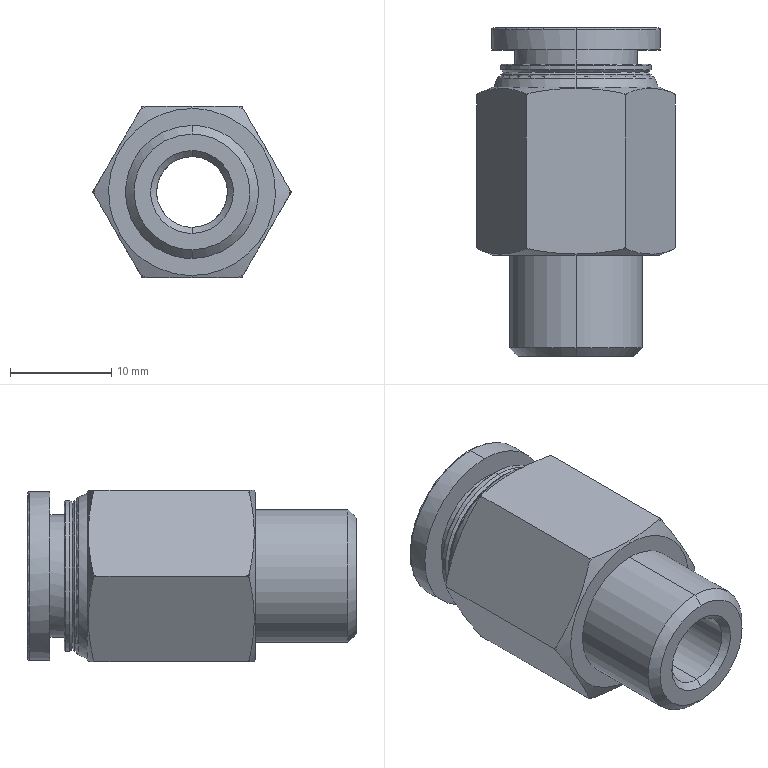Part | SolidWorks | features BaseBody 1 | 1 solid | 62 faces | box 19.63 x 32.5 x 17 mm | volume 4456 mm3 | torus 18 | cone 16 | cylinder 14 | plane 14 | commonest cylinder face diameters 14.9 x4 7 x2 10 x2 12.1 x2 13.157 x2 16.7 x2